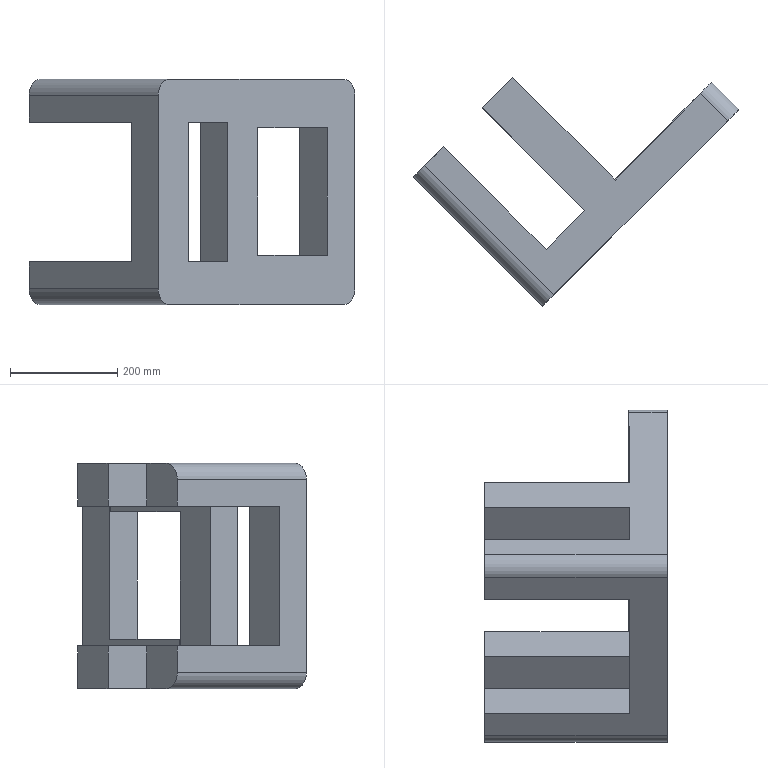Part | SolidWorks | 1 solid | 37 faces | box 606.344 x 425.772 x 420 mm | volume 17162651 mm3 | plane 33 | cylinder 4 | commonest cylinder face diameters 60 x4
STEP:
#1=CARTESIAN_POINT('',(51.005,517.696,-979.42));
#2=VERTEX_POINT('',#1);
#3=CARTESIAN_POINT('',(-139.914,708.614,-979.42));
#4=VERTEX_POINT('',#3);
#5=CARTESIAN_POINT('',(51.005,517.696,-979.42));
#6=DIRECTION('',(-0.7071,0.7071,0.));
#7=VECTOR('',#6,1000.);
#8=LINE('',#5,#7);
#9=EDGE_CURVE('',#2,#4,#8,.T.);
#10=ORIENTED_EDGE('',*,*,#9,.T.);
#11=CARTESIAN_POINT('',(-139.914,708.614,-899.42));
#12=VERTEX_POINT('',#11);
#13=CARTESIAN_POINT('',(-139.914,708.614,-899.42));
#14=DIRECTION('',(0.,0.,-1.));
#15=VECTOR('',#14,1000.);
#16=LINE('',#13,#15);
#17=EDGE_CURVE('',#12,#4,#16,.T.);
#18=ORIENTED_EDGE('',*,*,#17,.F.);
#19=CARTESIAN_POINT('',(51.005,517.696,-899.42));
#20=VERTEX_POINT('',#19);
#21=CARTESIAN_POINT('',(51.005,517.696,-899.42));
#22=DIRECTION('',(-0.7071,0.7071,0.));
#23=VECTOR('',#22,1000.);
#24=LINE('',#21,#23);
#25=EDGE_CURVE('',#20,#12,#24,.T.);
#26=ORIENTED_EDGE('',*,*,#25,.F.);
#27=CARTESIAN_POINT('',(51.005,517.696,-899.42));
#28=DIRECTION('',(0.,0.,-1.));
#29=VECTOR('',#28,1000.);
#30=LINE('',#27,#29);
#31=EDGE_CURVE('',#20,#2,#30,.T.);
#32=ORIENTED_EDGE('',*,*,#31,.T.);
#33=EDGE_LOOP('',(#10,#18,#26,#32));
#34=FACE_OUTER_BOUND('',#33,.T.);
#35=CARTESIAN_POINT('',(107.574,461.127,-1239.42));
#36=DIRECTION('',(0.7071,0.7071,0.));
#37=DIRECTION('',(0.,0.,-1.));
#38=AXIS2_PLACEMENT_3D('',#35,#36,#37);
#39=PLANE('',#38);
#40=ADVANCED_FACE('',(#34),#39,.T.);
#41=CARTESIAN_POINT('',(-196.482,652.046,-979.42));
#42=VERTEX_POINT('',#41);
#43=CARTESIAN_POINT('',(-139.914,708.614,-979.42));
#44=DIRECTION('',(-0.7071,-0.7071,0.));
#45=VECTOR('',#44,1000.);
#46=LINE('',#43,#45);
#47=EDGE_CURVE('',#4,#42,#46,.T.);
#48=ORIENTED_EDGE('',*,*,#47,.T.);
#49=CARTESIAN_POINT('',(-196.482,652.046,-899.42));
#50=VERTEX_POINT('',#49);
#51=CARTESIAN_POINT('',(-196.482,652.046,-979.42));
#52=DIRECTION('',(0.,0.,1.));
#53=VECTOR('',#52,1000.);
#54=LINE('',#51,#53);
#55=EDGE_CURVE('',#42,#50,#54,.T.);
#56=ORIENTED_EDGE('',*,*,#55,.T.);
#57=CARTESIAN_POINT('',(-196.482,652.046,-899.42));
#58=DIRECTION('',(0.7071,0.7071,0.));
#59=VECTOR('',#58,1000.);
#60=LINE('',#57,#59);
#61=EDGE_CURVE('',#50,#12,#60,.T.);
#62=ORIENTED_EDGE('',*,*,#61,.T.);
#63=ORIENTED_EDGE('',*,*,#17,.T.);
#64=EDGE_LOOP('',(#48,#56,#62,#63));
#65=FACE_OUTER_BOUND('',#64,.T.);
#66=CARTESIAN_POINT('',(-424.264,424.264,0.));
#67=DIRECTION('',(-0.7071,0.7071,0.));
#68=DIRECTION('',(-0.7071,-0.7071,0.));
#69=AXIS2_PLACEMENT_3D('',#66,#67,#68);
#70=PLANE('',#69);
#71=ADVANCED_FACE('',(#65),#70,.T.);
#72=CARTESIAN_POINT('',(-325.269,523.259,-979.42));
#73=VERTEX_POINT('',#72);
#74=CARTESIAN_POINT('',(-325.269,523.259,-929.42));
#75=VERTEX_POINT('',#74);
#76=CARTESIAN_POINT('',(-325.269,523.259,-979.42));
#77=DIRECTION('',(0.,0.,1.));
#78=VECTOR('',#77,1000.);
#79=LINE('',#76,#78);
#80=EDGE_CURVE('',#73,#75,#79,.T.);
#81=ORIENTED_EDGE('',*,*,#80,.T.);
#82=CARTESIAN_POINT('',(-304.056,544.472,-899.42));
#83=VERTEX_POINT('',#82);
#84=CARTESIAN_POINT('',(-304.056,544.472,-929.42));
#85=DIRECTION('',(-0.7071,0.7071,0.));
#86=DIRECTION('',(-0.7071,-0.7071,0.));
#87=AXIS2_PLACEMENT_3D('',#84,#85,#86);
#88=CIRCLE('',#87,30.);
#89=EDGE_CURVE('',#75,#83,#88,.T.);
#90=ORIENTED_EDGE('',*,*,#89,.T.);
#91=CARTESIAN_POINT('',(-268.701,579.828,-899.42));
#92=VERTEX_POINT('',#91);
#93=CARTESIAN_POINT('',(-325.269,523.259,-899.42));
#94=DIRECTION('',(0.7071,0.7071,0.));
#95=VECTOR('',#94,1000.);
#96=LINE('',#93,#95);
#97=EDGE_CURVE('',#83,#92,#96,.T.);
#98=ORIENTED_EDGE('',*,*,#97,.T.);
#99=CARTESIAN_POINT('',(-268.701,579.828,-979.42));
#100=VERTEX_POINT('',#99);
#101=CARTESIAN_POINT('',(-268.701,579.828,-899.42));
#102=DIRECTION('',(0.,0.,-1.));
#103=VECTOR('',#102,1000.);
#104=LINE('',#101,#103);
#105=EDGE_CURVE('',#92,#100,#104,.T.);
#106=ORIENTED_EDGE('',*,*,#105,.T.);
#107=CARTESIAN_POINT('',(-268.701,579.828,-979.42));
#108=DIRECTION('',(-0.7071,-0.7071,0.));
#109=VECTOR('',#108,1000.);
#110=LINE('',#107,#109);
#111=EDGE_CURVE('',#100,#73,#110,.T.);
#112=ORIENTED_EDGE('',*,*,#111,.T.);
#113=EDGE_LOOP('',(#81,#90,#98,#106,#112));
#114=FACE_OUTER_BOUND('',#113,.T.);
#115=CARTESIAN_POINT('',(-424.264,424.264,0.));
#116=DIRECTION('',(-0.7071,0.7071,0.));
#117=DIRECTION('',(-0.7071,-0.7071,0.));
#118=AXIS2_PLACEMENT_3D('',#115,#116,#117);
#119=PLANE('',#118);
#120=ADVANCED_FACE('',(#114),#119,.T.);
#121=CARTESIAN_POINT('',(-77.782,388.909,-979.42));
#122=VERTEX_POINT('',#121);
#123=CARTESIAN_POINT('',(-77.782,388.909,-979.42));
#124=DIRECTION('',(-0.7071,0.7071,0.));
#125=VECTOR('',#124,1000.);
#126=LINE('',#123,#125);
#127=EDGE_CURVE('',#122,#100,#126,.T.);
#128=ORIENTED_EDGE('',*,*,#127,.T.);
#129=ORIENTED_EDGE('',*,*,#105,.F.);
#130=CARTESIAN_POINT('',(-77.782,388.909,-899.42));
#131=VERTEX_POINT('',#130);
#132=CARTESIAN_POINT('',(-77.782,388.909,-899.42));
#133=DIRECTION('',(-0.7071,0.7071,0.));
#134=VECTOR('',#133,1000.);
#135=LINE('',#132,#134);
#136=EDGE_CURVE('',#131,#92,#135,.T.);
#137=ORIENTED_EDGE('',*,*,#136,.F.);
#138=CARTESIAN_POINT('',(-77.782,388.909,-899.42));
#139=DIRECTION('',(0.,0.,-1.));
#140=VECTOR('',#139,1000.);
#141=LINE('',#138,#140);
#142=EDGE_CURVE('',#131,#122,#141,.T.);
#143=ORIENTED_EDGE('',*,*,#142,.T.);
#144=EDGE_LOOP('',(#128,#129,#137,#143));
#145=FACE_OUTER_BOUND('',#144,.T.);
#146=CARTESIAN_POINT('',(-28.284,339.411,-899.42));
#147=DIRECTION('',(0.7071,0.7071,0.));
#148=DIRECTION('',(0.,0.,-1.));
#149=AXIS2_PLACEMENT_3D('',#146,#147,#148);
#150=PLANE('',#149);
#151=ADVANCED_FACE('',(#145),#150,.T.);
#152=CARTESIAN_POINT('',(-134.35,332.34,-979.42));
#153=VERTEX_POINT('',#152);
#154=CARTESIAN_POINT('',(-77.782,388.909,-979.42));
#155=DIRECTION('',(-0.7071,-0.7071,0.));
#156=VECTOR('',#155,1000.);
#157=LINE('',#154,#156);
#158=EDGE_CURVE('',#122,#153,#157,.T.);
#159=ORIENTED_EDGE('',*,*,#158,.T.);
#160=CARTESIAN_POINT('',(-134.35,332.34,-979.42));
#161=DIRECTION('',(-0.7071,0.7071,0.));
#162=VECTOR('',#161,1000.);
#163=LINE('',#160,#162);
#164=EDGE_CURVE('',#153,#73,#163,.T.);
#165=ORIENTED_EDGE('',*,*,#164,.T.);
#166=ORIENTED_EDGE('',*,*,#111,.F.);
#167=ORIENTED_EDGE('',*,*,#127,.F.);
#168=EDGE_LOOP('',(#159,#165,#166,#167));
#169=FACE_OUTER_BOUND('',#168,.T.);
#170=CARTESIAN_POINT('',(-28.284,339.411,-979.42));
#171=DIRECTION('',(0.,0.,-1.));
#172=DIRECTION('',(-0.7071,-0.7071,0.));
#173=AXIS2_PLACEMENT_3D('',#170,#171,#172);
#174=PLANE('',#173);
#175=ADVANCED_FACE('',(#169),#174,.T.);
#176=CARTESIAN_POINT('',(-134.35,332.34,-1239.42));
#177=VERTEX_POINT('',#176);
#178=CARTESIAN_POINT('',(-77.782,388.909,-1239.42));
#179=VERTEX_POINT('',#178);
#180=CARTESIAN_POINT('',(-134.35,332.34,-1239.42));
#181=DIRECTION('',(0.7071,0.7071,0.));
#182=VECTOR('',#181,1000.);
#183=LINE('',#180,#182);
#184=EDGE_CURVE('',#177,#179,#183,.T.);
#185=ORIENTED_EDGE('',*,*,#184,.F.);
#186=CARTESIAN_POINT('',(-134.35,332.34,-1239.42));
#187=DIRECTION('',(0.,0.,1.));
#188=VECTOR('',#187,1000.);
#189=LINE('',#186,#188);
#190=EDGE_CURVE('',#177,#153,#189,.T.);
#191=ORIENTED_EDGE('',*,*,#190,.T.);
#192=ORIENTED_EDGE('',*,*,#158,.F.);
#193=CARTESIAN_POINT('',(-77.782,388.909,-1239.42));
#194=DIRECTION('',(0.,0.,1.));
#195=VECTOR('',#194,1000.);
#196=LINE('',#193,#195);
#197=EDGE_CURVE('',#179,#122,#196,.T.);
#198=ORIENTED_EDGE('',*,*,#197,.F.);
#199=EDGE_LOOP('',(#185,#191,#192,#198));
#200=FACE_OUTER_BOUND('',#199,.T.);
#201=CARTESIAN_POINT('',(-134.35,332.34,-1319.42));
#202=DIRECTION('',(-0.7071,0.7071,0.));
#203=DIRECTION('',(0.7071,0.7071,0.));
#204=AXIS2_PLACEMENT_3D('',#201,#202,#203);
#205=PLANE('',#204);
#206=ADVANCED_FACE('',(#200),#205,.T.);
#207=CARTESIAN_POINT('',(43.934,411.63,-979.42));
#208=VERTEX_POINT('',#207);
#209=CARTESIAN_POINT('',(-5.563,461.127,-979.42));
#210=VERTEX_POINT('',#209);
#211=CARTESIAN_POINT('',(43.934,411.63,-979.42));
#212=DIRECTION('',(-0.7071,0.7071,0.));
#213=VECTOR('',#212,1000.);
#214=LINE('',#211,#213);
#215=EDGE_CURVE('',#208,#210,#214,.T.);
#216=ORIENTED_EDGE('',*,*,#215,.T.);
#217=CARTESIAN_POINT('',(-5.563,461.127,-1239.42));
#218=VERTEX_POINT('',#217);
#219=CARTESIAN_POINT('',(-5.563,461.127,-1239.42));
#220=DIRECTION('',(0.,0.,1.));
#221=VECTOR('',#220,1000.);
#222=LINE('',#219,#221);
#223=EDGE_CURVE('',#218,#210,#222,.T.);
#224=ORIENTED_EDGE('',*,*,#223,.F.);
#225=CARTESIAN_POINT('',(43.934,411.63,-1239.42));
#226=VERTEX_POINT('',#225);
#227=CARTESIAN_POINT('',(43.934,411.63,-1239.42));
#228=DIRECTION('',(-0.7071,0.7071,0.));
#229=VECTOR('',#228,1000.);
#230=LINE('',#227,#229);
#231=EDGE_CURVE('',#226,#218,#230,.T.);
#232=ORIENTED_EDGE('',*,*,#231,.F.);
#233=CARTESIAN_POINT('',(43.934,411.63,-1239.42));
#234=DIRECTION('',(0.,0.,1.));
#235=VECTOR('',#234,1000.);
#236=LINE('',#233,#235);
#237=EDGE_CURVE('',#226,#208,#236,.T.);
#238=ORIENTED_EDGE('',*,*,#237,.T.);
#239=EDGE_LOOP('',(#216,#224,#232,#238));
#240=FACE_OUTER_BOUND('',#239,.T.);
#241=CARTESIAN_POINT('',(51.005,404.558,-1319.42));
#242=DIRECTION('',(-0.7071,-0.7071,0.));
#243=DIRECTION('',(0.,0.,1.));
#244=AXIS2_PLACEMENT_3D('',#241,#242,#243);
#245=PLANE('',#244);
#246=ADVANCED_FACE('',(#240),#245,.T.);
#247=CARTESIAN_POINT('',(-28.284,339.411,-979.42));
#248=VERTEX_POINT('',#247);
#249=CARTESIAN_POINT('',(-28.284,339.411,-979.42));
#250=DIRECTION('',(-0.7071,0.7071,0.));
#251=VECTOR('',#250,1000.);
#252=LINE('',#249,#251);
#253=EDGE_CURVE('',#248,#122,#252,.T.);
#254=ORIENTED_EDGE('',*,*,#253,.T.);
#255=CARTESIAN_POINT('',(-77.782,388.909,-979.42));
#256=DIRECTION('',(0.7071,0.7071,0.));
#257=VECTOR('',#256,1000.);
#258=LINE('',#255,#257);
#259=EDGE_CURVE('',#122,#210,#258,.T.);
#260=ORIENTED_EDGE('',*,*,#259,.T.);
#261=ORIENTED_EDGE('',*,*,#215,.F.);
#262=CARTESIAN_POINT('',(43.934,411.63,-979.42));
#263=DIRECTION('',(-0.7071,-0.7071,0.));
#264=VECTOR('',#263,1000.);
#265=LINE('',#262,#264);
#266=EDGE_CURVE('',#208,#248,#265,.T.);
#267=ORIENTED_EDGE('',*,*,#266,.T.);
#268=EDGE_LOOP('',(#254,#260,#261,#267));
#269=FACE_OUTER_BOUND('',#268,.T.);
#270=CARTESIAN_POINT('',(-134.35,332.34,-979.42));
#271=DIRECTION('',(0.,0.,-1.));
#272=DIRECTION('',(0.7071,-0.7071,0.));
#273=AXIS2_PLACEMENT_3D('',#270,#271,#272);
#274=PLANE('',#273);
#275=ADVANCED_FACE('',(#269),#274,.T.);
#276=CARTESIAN_POINT('',(-28.284,339.411,-1239.42));
#277=VERTEX_POINT('',#276);
#278=CARTESIAN_POINT('',(-28.284,339.411,-1239.42));
#279=DIRECTION('',(-0.7071,0.7071,0.));
#280=VECTOR('',#279,1000.);
#281=LINE('',#278,#280);
#282=EDGE_CURVE('',#277,#179,#281,.T.);
#283=ORIENTED_EDGE('',*,*,#282,.T.);
#284=ORIENTED_EDGE('',*,*,#197,.T.);
#285=ORIENTED_EDGE('',*,*,#253,.F.);
#286=CARTESIAN_POINT('',(-28.284,339.411,-979.42));
#287=DIRECTION('',(0.,0.,-1.));
#288=VECTOR('',#287,1000.);
#289=LINE('',#286,#288);
#290=EDGE_CURVE('',#248,#277,#289,.T.);
#291=ORIENTED_EDGE('',*,*,#290,.T.);
#292=EDGE_LOOP('',(#283,#284,#285,#291));
#293=FACE_OUTER_BOUND('',#292,.T.);
#294=CARTESIAN_POINT('',(-28.284,339.411,-899.42));
#295=DIRECTION('',(0.7071,0.7071,0.));
#296=DIRECTION('',(0.,0.,-1.));
#297=AXIS2_PLACEMENT_3D('',#294,#295,#296);
#298=PLANE('',#297);
#299=ADVANCED_FACE('',(#293),#298,.T.);
#300=ORIENTED_EDGE('',*,*,#231,.T.);
#301=CARTESIAN_POINT('',(-77.782,388.909,-1239.42));
#302=DIRECTION('',(0.7071,0.7071,0.));
#303=VECTOR('',#302,1000.);
#304=LINE('',#301,#303);
#305=EDGE_CURVE('',#179,#218,#304,.T.);
#306=ORIENTED_EDGE('',*,*,#305,.F.);
#307=ORIENTED_EDGE('',*,*,#282,.F.);
#308=CARTESIAN_POINT('',(43.934,411.63,-1239.42));
#309=DIRECTION('',(-0.7071,-0.7071,0.));
#310=VECTOR('',#309,1000.);
#311=LINE('',#308,#310);
#312=EDGE_CURVE('',#226,#277,#311,.T.);
#313=ORIENTED_EDGE('',*,*,#312,.F.);
#314=EDGE_LOOP('',(#300,#306,#307,#313));
#315=FACE_OUTER_BOUND('',#314,.T.);
#316=CARTESIAN_POINT('',(-77.782,275.772,-1239.42));
#317=DIRECTION('',(0.,0.,1.));
#318=DIRECTION('',(-0.7071,0.7071,0.));
#319=AXIS2_PLACEMENT_3D('',#316,#317,#318);
#320=PLANE('',#319);
#321=ADVANCED_FACE('',(#315),#320,.T.);
#322=CARTESIAN_POINT('',(49.428,519.273,-1239.42));
#323=VERTEX_POINT('',#322);
#324=CARTESIAN_POINT('',(-139.914,708.614,-1239.42));
#325=VERTEX_POINT('',#324);
#326=CARTESIAN_POINT('',(49.428,519.273,-1239.42));
#327=DIRECTION('',(-0.7071,0.7071,0.));
#328=VECTOR('',#327,1000.);
#329=LINE('',#326,#328);
#330=EDGE_CURVE('',#323,#325,#329,.T.);
#331=ORIENTED_EDGE('',*,*,#330,.T.);
#332=CARTESIAN_POINT('',(-196.482,652.046,-1239.42));
#333=VERTEX_POINT('',#332);
#334=CARTESIAN_POINT('',(-196.482,652.046,-1239.42));
#335=DIRECTION('',(0.7071,0.7071,0.));
#336=VECTOR('',#335,1000.);
#337=LINE('',#334,#336);
#338=EDGE_CURVE('',#333,#325,#337,.T.);
#339=ORIENTED_EDGE('',*,*,#338,.F.);
#340=CARTESIAN_POINT('',(-5.563,461.127,-1239.42));
#341=DIRECTION('',(-0.7071,0.7071,0.));
#342=VECTOR('',#341,1000.);
#343=LINE('',#340,#342);
#344=EDGE_CURVE('',#218,#333,#343,.T.);
#345=ORIENTED_EDGE('',*,*,#344,.F.);
#346=CARTESIAN_POINT('',(51.005,517.696,-1239.42));
#347=VERTEX_POINT('',#346);
#348=CARTESIAN_POINT('',(-5.563,461.127,-1239.42));
#349=DIRECTION('',(0.7071,0.7071,0.));
#350=VECTOR('',#349,1000.);
#351=LINE('',#348,#350);
#352=EDGE_CURVE('',#218,#347,#351,.T.);
#353=ORIENTED_EDGE('',*,*,#352,.T.);
#354=CARTESIAN_POINT('',(51.005,517.696,-1239.42));
#355=DIRECTION('',(-0.7071,0.7071,0.));
#356=VECTOR('',#355,1000.);
#357=LINE('',#354,#356);
#358=EDGE_CURVE('',#347,#323,#357,.T.);
#359=ORIENTED_EDGE('',*,*,#358,.T.);
#360=EDGE_LOOP('',(#331,#339,#345,#353,#359));
#361=FACE_OUTER_BOUND('',#360,.T.);
#362=CARTESIAN_POINT('',(51.005,404.558,-1239.42));
#363=DIRECTION('',(0.,0.,1.));
#364=DIRECTION('',(0.7071,0.7071,0.));
#365=AXIS2_PLACEMENT_3D('',#362,#363,#364);
#366=PLANE('',#365);
#367=ADVANCED_FACE('',(#361),#366,.T.);
#368=CARTESIAN_POINT('',(51.005,517.696,-1227.42));
#369=VERTEX_POINT('',#368);
#370=CARTESIAN_POINT('',(51.005,517.696,-1227.42));
#371=DIRECTION('',(0.,0.,-1.));
#372=VECTOR('',#371,1000.);
#373=LINE('',#370,#372);
#374=EDGE_CURVE('',#369,#347,#373,.T.);
#375=ORIENTED_EDGE('',*,*,#374,.F.);
#376=CARTESIAN_POINT('',(49.428,519.273,-1227.42));
#377=VERTEX_POINT('',#376);
#378=CARTESIAN_POINT('',(49.428,519.273,-1227.42));
#379=DIRECTION('',(0.7071,-0.7071,0.));
#380=VECTOR('',#379,1000.);
#381=LINE('',#378,#380);
#382=EDGE_CURVE('',#377,#369,#381,.T.);
#383=ORIENTED_EDGE('',*,*,#382,.F.);
#384=CARTESIAN_POINT('',(49.428,519.273,-1239.42));
#385=DIRECTION('',(0.,0.,1.));
#386=VECTOR('',#385,1000.);
#387=LINE('',#384,#386);
#388=EDGE_CURVE('',#323,#377,#387,.T.);
#389=ORIENTED_EDGE('',*,*,#388,.F.);
#390=ORIENTED_EDGE('',*,*,#358,.F.);
#391=EDGE_LOOP('',(#375,#383,#389,#390));
#392=FACE_OUTER_BOUND('',#391,.T.);
#393=CARTESIAN_POINT('',(107.574,461.127,0.));
#394=DIRECTION('',(0.7071,0.7071,0.));
#395=DIRECTION('',(0.,0.,1.));
#396=AXIS2_PLACEMENT_3D('',#393,#394,#395);
#397=PLANE('',#396);
#398=ADVANCED_FACE('',(#392),#397,.F.);
#399=CARTESIAN_POINT('',(100.503,468.198,-1227.42));
#400=VERTEX_POINT('',#399);
#401=CARTESIAN_POINT('',(230.,597.696,-1227.42));
#402=VERTEX_POINT('',#401);
#403=CARTESIAN_POINT('',(100.503,468.198,-1227.42));
#404=DIRECTION('',(0.7071,0.7071,0.));
#405=VECTOR('',#404,1000.);
#406=LINE('',#403,#405);
#407=EDGE_CURVE('',#400,#402,#406,.T.);
#408=ORIENTED_EDGE('',*,*,#407,.T.);
#409=CARTESIAN_POINT('',(178.925,648.77,-1227.42));
#410=VERTEX_POINT('',#409);
#411=CARTESIAN_POINT('',(178.925,648.77,-1227.42));
#412=DIRECTION('',(0.7071,-0.7071,0.));
#413=VECTOR('',#412,1000.);
#414=LINE('',#411,#413);
#415=EDGE_CURVE('',#410,#402,#414,.T.);
#416=ORIENTED_EDGE('',*,*,#415,.F.);
#417=CARTESIAN_POINT('',(49.428,519.273,-1227.42));
#418=DIRECTION('',(0.7071,0.7071,0.));
#419=VECTOR('',#418,1000.);
#420=LINE('',#417,#419);
#421=EDGE_CURVE('',#377,#410,#420,.T.);
#422=ORIENTED_EDGE('',*,*,#421,.F.);
#423=ORIENTED_EDGE('',*,*,#382,.T.);
#424=CARTESIAN_POINT('',(51.005,517.696,-1227.42));
#425=DIRECTION('',(0.7071,-0.7071,0.));
#426=VECTOR('',#425,1000.);
#427=LINE('',#424,#426);
#428=EDGE_CURVE('',#369,#400,#427,.T.);
#429=ORIENTED_EDGE('',*,*,#428,.T.);
#430=EDGE_LOOP('',(#408,#416,#422,#423,#429));
#431=FACE_OUTER_BOUND('',#430,.T.);
#432=CARTESIAN_POINT('',(49.428,519.273,-1227.42));
#433=DIRECTION('',(0.,0.,1.));
#434=DIRECTION('',(0.7071,-0.7071,0.));
#435=AXIS2_PLACEMENT_3D('',#432,#433,#434);
#436=PLANE('',#435);
#437=ADVANCED_FACE('',(#431),#436,.T.);
#438=CARTESIAN_POINT('',(230.,699.845,-1289.42));
#439=VERTEX_POINT('',#438);
#440=CARTESIAN_POINT('',(230.,699.845,-929.42));
#441=VERTEX_POINT('',#440);
#442=CARTESIAN_POINT('',(230.,699.845,-1319.42));
#443=DIRECTION('',(0.,0.,1.));
#444=VECTOR('',#443,1000.);
#445=LINE('',#442,#444);
#446=EDGE_CURVE('',#439,#441,#445,.T.);
#447=ORIENTED_EDGE('',*,*,#446,.F.);
#448=CARTESIAN_POINT('',(208.787,678.632,-1319.42));
#449=VERTEX_POINT('',#448);
#450=CARTESIAN_POINT('',(208.787,678.632,-1289.42));
#451=DIRECTION('',(-0.7071,0.7071,0.));
#452=DIRECTION('',(-0.7071,-0.7071,0.));
#453=AXIS2_PLACEMENT_3D('',#450,#451,#452);
#454=CIRCLE('',#453,30.);
#455=EDGE_CURVE('',#439,#449,#454,.T.);
#456=ORIENTED_EDGE('',*,*,#455,.T.);
#457=CARTESIAN_POINT('',(49.428,519.273,-1319.42));
#458=VERTEX_POINT('',#457);
#459=CARTESIAN_POINT('',(49.428,519.273,-1319.42));
#460=DIRECTION('',(0.7071,0.7071,0.));
#461=VECTOR('',#460,1000.);
#462=LINE('',#459,#461);
#463=EDGE_CURVE('',#458,#449,#462,.T.);
#464=ORIENTED_EDGE('',*,*,#463,.F.);
#465=CARTESIAN_POINT('',(49.428,519.273,-1319.42));
#466=DIRECTION('',(0.,0.,1.));
#467=VECTOR('',#466,1000.);
#468=LINE('',#465,#467);
#469=EDGE_CURVE('',#458,#323,#468,.T.);
#470=ORIENTED_EDGE('',*,*,#469,.T.);
#471=ORIENTED_EDGE('',*,*,#388,.T.);
#472=ORIENTED_EDGE('',*,*,#421,.T.);
#473=CARTESIAN_POINT('',(178.925,648.77,-899.42));
#474=VERTEX_POINT('',#473);
#475=CARTESIAN_POINT('',(178.925,648.77,-1227.42));
#476=DIRECTION('',(0.,0.,1.));
#477=VECTOR('',#476,1000.);
#478=LINE('',#475,#477);
#479=EDGE_CURVE('',#410,#474,#478,.T.);
#480=ORIENTED_EDGE('',*,*,#479,.T.);
#481=CARTESIAN_POINT('',(208.787,678.632,-899.42));
#482=VERTEX_POINT('',#481);
#483=CARTESIAN_POINT('',(178.925,648.77,-899.42));
#484=DIRECTION('',(0.7071,0.7071,0.));
#485=VECTOR('',#484,1000.);
#486=LINE('',#483,#485);
#487=EDGE_CURVE('',#474,#482,#486,.T.);
#488=ORIENTED_EDGE('',*,*,#487,.T.);
#489=CARTESIAN_POINT('',(208.787,678.632,-929.42));
#490=DIRECTION('',(-0.7071,0.7071,0.));
#491=DIRECTION('',(-0.7071,-0.7071,0.));
#492=AXIS2_PLACEMENT_3D('',#489,#490,#491);
#493=CIRCLE('',#492,30.);
#494=EDGE_CURVE('',#482,#441,#493,.T.);
#495=ORIENTED_EDGE('',*,*,#494,.T.);
#496=EDGE_LOOP('',(#447,#456,#464,#470,#471,#472,#480,#488,#495));
#497=FACE_OUTER_BOUND('',#496,.T.);
#498=CARTESIAN_POINT('',(49.428,519.273,-1319.42));
#499=DIRECTION('',(-0.7071,0.7071,0.));
#500=DIRECTION('',(0.,0.,1.));
#501=AXIS2_PLACEMENT_3D('',#498,#499,#500);
#502=PLANE('',#501);
#503=ADVANCED_FACE('',(#497),#502,.T.);
#504=CARTESIAN_POINT('',(-139.914,708.614,-1319.42));
#505=VERTEX_POINT('',#504);
#506=CARTESIAN_POINT('',(49.428,519.273,-1319.42));
#507=DIRECTION('',(-0.7071,0.7071,0.));
#508=VECTOR('',#507,1000.);
#509=LINE('',#506,#508);
#510=EDGE_CURVE('',#458,#505,#509,.T.);
#511=ORIENTED_EDGE('',*,*,#510,.T.);
#512=CARTESIAN_POINT('',(-139.914,708.614,-1239.42));
#513=DIRECTION('',(0.,0.,-1.));
#514=VECTOR('',#513,1000.);
#515=LINE('',#512,#514);
#516=EDGE_CURVE('',#325,#505,#515,.T.);
#517=ORIENTED_EDGE('',*,*,#516,.F.);
#518=ORIENTED_EDGE('',*,*,#330,.F.);
#519=ORIENTED_EDGE('',*,*,#469,.F.);
#520=EDGE_LOOP('',(#511,#517,#518,#519));
#521=FACE_OUTER_BOUND('',#520,.T.);
#522=CARTESIAN_POINT('',(107.574,461.127,-1239.42));
#523=DIRECTION('',(0.7071,0.7071,0.));
#524=DIRECTION('',(0.,0.,-1.));
#525=AXIS2_PLACEMENT_3D('',#522,#523,#524);
#526=PLANE('',#525);
#527=ADVANCED_FACE('',(#521),#526,.T.);
#528=CARTESIAN_POINT('',(-196.482,652.046,-1319.42));
#529=VERTEX_POINT('',#528);
#530=CARTESIAN_POINT('',(-196.482,652.046,-1319.42));
#531=DIRECTION('',(0.,0.,1.));
#532=VECTOR('',#531,1000.);
#533=LINE('',#530,#532);
#534=EDGE_CURVE('',#529,#333,#533,.T.);
#535=ORIENTED_EDGE('',*,*,#534,.T.);
#536=ORIENTED_EDGE('',*,*,#338,.T.);
#537=ORIENTED_EDGE('',*,*,#516,.T.);
#538=CARTESIAN_POINT('',(-139.914,708.614,-1319.42));
#539=DIRECTION('',(-0.7071,-0.7071,0.));
#540=VECTOR('',#539,1000.);
#541=LINE('',#538,#540);
#542=EDGE_CURVE('',#505,#529,#541,.T.);
#543=ORIENTED_EDGE('',*,*,#542,.T.);
#544=EDGE_LOOP('',(#535,#536,#537,#543));
#545=FACE_OUTER_BOUND('',#544,.T.);
#546=CARTESIAN_POINT('',(-424.264,424.264,0.));
#547=DIRECTION('',(-0.7071,0.7071,0.));
#548=DIRECTION('',(-0.7071,-0.7071,0.));
#549=AXIS2_PLACEMENT_3D('',#546,#547,#548);
#550=PLANE('',#549);
#551=ADVANCED_FACE('',(#545),#550,.T.);
#552=ORIENTED_EDGE('',*,*,#344,.T.);
#553=ORIENTED_EDGE('',*,*,#534,.F.);
#554=CARTESIAN_POINT('',(-5.563,461.127,-1319.42));
#555=VERTEX_POINT('',#554);
#556=CARTESIAN_POINT('',(-5.563,461.127,-1319.42));
#557=DIRECTION('',(-0.7071,0.7071,0.));
#558=VECTOR('',#557,1000.);
#559=LINE('',#556,#558);
#560=EDGE_CURVE('',#555,#529,#559,.T.);
#561=ORIENTED_EDGE('',*,*,#560,.F.);
#562=CARTESIAN_POINT('',(-5.563,461.127,-1319.42));
#563=DIRECTION('',(0.,0.,1.));
#564=VECTOR('',#563,1000.);
#565=LINE('',#562,#564);
#566=EDGE_CURVE('',#555,#218,#565,.T.);
#567=ORIENTED_EDGE('',*,*,#566,.T.);
#568=EDGE_LOOP('',(#552,#553,#561,#567));
#569=FACE_OUTER_BOUND('',#568,.T.);
#570=CARTESIAN_POINT('',(51.005,404.558,-1319.42));
#571=DIRECTION('',(-0.7071,-0.7071,0.));
#572=DIRECTION('',(0.,0.,1.));
#573=AXIS2_PLACEMENT_3D('',#570,#571,#572);
#574=PLANE('',#573);
#575=ADVANCED_FACE('',(#569),#574,.T.);
#576=CARTESIAN_POINT('',(-77.782,388.909,-1319.42));
#577=VERTEX_POINT('',#576);
#578=CARTESIAN_POINT('',(-77.782,388.909,-1319.42));
#579=DIRECTION('',(0.7071,0.7071,0.));
#580=VECTOR('',#579,1000.);
#581=LINE('',#578,#580);
#582=EDGE_CURVE('',#577,#555,#581,.T.);
#583=ORIENTED_EDGE('',*,*,#582,.F.);
#584=CARTESIAN_POINT('',(-77.782,388.909,-1319.42));
#585=DIRECTION('',(0.,0.,1.));
#586=VECTOR('',#585,1000.);
#587=LINE('',#584,#586);
#588=EDGE_CURVE('',#577,#179,#587,.T.);
#589=ORIENTED_EDGE('',*,*,#588,.T.);
#590=ORIENTED_EDGE('',*,*,#305,.T.);
#591=ORIENTED_EDGE('',*,*,#566,.F.);
#592=EDGE_LOOP('',(#583,#589,#590,#591));
#593=FACE_OUTER_BOUND('',#592,.T.);
#594=CARTESIAN_POINT('',(-134.35,332.34,-1239.42));
#595=DIRECTION('',(-0.7071,0.7071,0.));
#596=DIRECTION('',(0.,0.,-1.));
#597=AXIS2_PLACEMENT_3D('',#594,#595,#596);
#598=PLANE('',#597);
#599=ADVANCED_FACE('',(#593),#598,.T.);
#600=CARTESIAN_POINT('',(-268.701,579.828,-1319.42));
#601=VERTEX_POINT('',#600);
#602=CARTESIAN_POINT('',(-268.701,579.828,-1319.42));
#603=DIRECTION('',(0.7071,-0.7071,0.));
#604=VECTOR('',#603,1000.);
#605=LINE('',#602,#604);
#606=EDGE_CURVE('',#601,#577,#605,.T.);
#607=ORIENTED_EDGE('',*,*,#606,.F.);
#608=CARTESIAN_POINT('',(-268.701,579.828,-1239.42));
#609=VERTEX_POINT('',#608);
#610=CARTESIAN_POINT('',(-268.701,579.828,-1239.42));
#611=DIRECTION('',(0.,0.,-1.));
#612=VECTOR('',#611,1000.);
#613=LINE('',#610,#612);
#614=EDGE_CURVE('',#609,#601,#613,.T.);
#615=ORIENTED_EDGE('',*,*,#614,.F.);
#616=CARTESIAN_POINT('',(-77.782,388.909,-1239.42));
#617=DIRECTION('',(-0.7071,0.7071,0.));
#618=VECTOR('',#617,1000.);
#619=LINE('',#616,#618);
#620=EDGE_CURVE('',#179,#609,#619,.T.);
#621=ORIENTED_EDGE('',*,*,#620,.F.);
#622=ORIENTED_EDGE('',*,*,#588,.F.);
#623=EDGE_LOOP('',(#607,#615,#621,#622));
#624=FACE_OUTER_BOUND('',#623,.T.);
#625=CARTESIAN_POINT('',(-28.284,339.411,-899.42));
#626=DIRECTION('',(0.7071,0.7071,0.));
#627=DIRECTION('',(0.,0.,-1.));
#628=AXIS2_PLACEMENT_3D('',#625,#626,#627);
#629=PLANE('',#628);
#630=ADVANCED_FACE('',(#624),#629,.T.);
#631=CARTESIAN_POINT('',(-325.269,523.259,-1239.42));
#632=VERTEX_POINT('',#631);
#633=CARTESIAN_POINT('',(-325.269,523.259,-1239.42));
#634=DIRECTION('',(0.7071,0.7071,0.));
#635=VECTOR('',#634,1000.);
#636=LINE('',#633,#635);
#637=EDGE_CURVE('',#632,#609,#636,.T.);
#638=ORIENTED_EDGE('',*,*,#637,.F.);
#639=CARTESIAN_POINT('',(-134.35,332.34,-1239.42));
#640=DIRECTION('',(-0.7071,0.7071,0.));
#641=VECTOR('',#640,1000.);
#642=LINE('',#639,#641);
#643=EDGE_CURVE('',#177,#632,#642,.T.);
#644=ORIENTED_EDGE('',*,*,#643,.F.);
#645=ORIENTED_EDGE('',*,*,#184,.T.);
#646=ORIENTED_EDGE('',*,*,#620,.T.);
#647=EDGE_LOOP('',(#638,#644,#645,#646));
#648=FACE_OUTER_BOUND('',#647,.T.);
#649=CARTESIAN_POINT('',(-84.853,282.843,-1239.42));
#650=DIRECTION('',(0.,0.,1.));
#651=DIRECTION('',(0.7071,0.7071,0.));
#652=AXIS2_PLACEMENT_3D('',#649,#650,#651);
#653=PLANE('',#652);
#654=ADVANCED_FACE('',(#648),#653,.T.);
#655=CARTESIAN_POINT('',(-304.056,544.472,-1319.42));
#656=VERTEX_POINT('',#655);
#657=CARTESIAN_POINT('',(-268.701,579.828,-1319.42));
#658=DIRECTION('',(-0.7071,-0.7071,0.));
#659=VECTOR('',#658,1000.);
#660=LINE('',#657,#659);
#661=EDGE_CURVE('',#601,#656,#660,.T.);
#662=ORIENTED_EDGE('',*,*,#661,.T.);
#663=CARTESIAN_POINT('',(-325.269,523.259,-1289.42));
#664=VERTEX_POINT('',#663);
#665=CARTESIAN_POINT('',(-304.056,544.472,-1289.42));
#666=DIRECTION('',(-0.7071,0.7071,0.));
#667=DIRECTION('',(-0.7071,-0.7071,0.));
#668=AXIS2_PLACEMENT_3D('',#665,#666,#667);
#669=CIRCLE('',#668,30.);
#670=EDGE_CURVE('',#656,#664,#669,.T.);
#671=ORIENTED_EDGE('',*,*,#670,.T.);
#672=CARTESIAN_POINT('',(-325.269,523.259,-1319.42));
#673=DIRECTION('',(0.,0.,1.));
#674=VECTOR('',#673,1000.);
#675=LINE('',#672,#674);
#676=EDGE_CURVE('',#664,#632,#675,.T.);
#677=ORIENTED_EDGE('',*,*,#676,.T.);
#678=ORIENTED_EDGE('',*,*,#637,.T.);
#679=ORIENTED_EDGE('',*,*,#614,.T.);
#680=EDGE_LOOP('',(#662,#671,#677,#678,#679));
#681=FACE_OUTER_BOUND('',#680,.T.);
#682=CARTESIAN_POINT('',(-424.264,424.264,0.));
#683=DIRECTION('',(-0.7071,0.7071,0.));
#684=DIRECTION('',(-0.7071,-0.7071,0.));
#685=AXIS2_PLACEMENT_3D('',#682,#683,#684);
#686=PLANE('',#685);
#687=ADVANCED_FACE('',(#681),#686,.T.);
#688=ORIENTED_EDGE('',*,*,#676,.F.);
#689=CARTESIAN_POINT('',(-84.853,282.843,-1289.42));
#690=VERTEX_POINT('',#689);
#691=CARTESIAN_POINT('',(-84.853,282.843,-1289.42));
#692=DIRECTION('',(0.7071,-0.7071,0.));
#693=VECTOR('',#692,1000.);
#694=LINE('',#691,#693);
#695=EDGE_CURVE('',#664,#690,#694,.T.);
#696=ORIENTED_EDGE('',*,*,#695,.T.);
#697=CARTESIAN_POINT('',(-84.853,282.843,-929.42));
#698=VERTEX_POINT('',#697);
#699=CARTESIAN_POINT('',(-84.853,282.843,-1319.42));
#700=DIRECTION('',(0.,0.,1.));
#701=VECTOR('',#700,1000.);
#702=LINE('',#699,#701);
#703=EDGE_CURVE('',#690,#698,#702,.T.);
#704=ORIENTED_EDGE('',*,*,#703,.T.);
#705=CARTESIAN_POINT('',(-84.853,282.843,-929.42));
#706=DIRECTION('',(-0.7071,0.7071,0.));
#707=VECTOR('',#706,1000.);
#708=LINE('',#705,#707);
#709=EDGE_CURVE('',#698,#75,#708,.T.);
#710=ORIENTED_EDGE('',*,*,#709,.T.);
#711=ORIENTED_EDGE('',*,*,#80,.F.);
#712=ORIENTED_EDGE('',*,*,#164,.F.);
#713=ORIENTED_EDGE('',*,*,#190,.F.);
#714=ORIENTED_EDGE('',*,*,#643,.T.);
#715=EDGE_LOOP('',(#688,#696,#704,#710,#711,#712,#713,#714));
#716=FACE_OUTER_BOUND('',#715,.T.);
#717=CARTESIAN_POINT('',(-84.853,282.843,-979.42));
#718=DIRECTION('',(-0.7071,-0.7071,0.));
#719=DIRECTION('',(0.,0.,1.));
#720=AXIS2_PLACEMENT_3D('',#717,#718,#719);
#721=PLANE('',#720);
#722=ADVANCED_FACE('',(#716),#721,.T.);
#723=ORIENTED_EDGE('',*,*,#97,.F.);
#724=CARTESIAN_POINT('',(-63.64,304.056,-899.42));
#725=VERTEX_POINT('',#724);
#726=CARTESIAN_POINT('',(-56.569,296.985,-899.42));
#727=DIRECTION('',(0.7071,-0.7071,0.));
#728=VECTOR('',#727,1000.);
#729=LINE('',#726,#728);
#730=EDGE_CURVE('',#83,#725,#729,.T.);
#731=ORIENTED_EDGE('',*,*,#730,.T.);
#732=CARTESIAN_POINT('',(259.862,627.557,-899.42));
#733=VERTEX_POINT('',#732);
#734=CARTESIAN_POINT('',(-84.853,282.843,-899.42));
#735=DIRECTION('',(0.7071,0.7071,0.));
#736=VECTOR('',#735,1000.);
#737=LINE('',#734,#736);
#738=EDGE_CURVE('',#725,#733,#737,.T.);
#739=ORIENTED_EDGE('',*,*,#738,.T.);
#740=CARTESIAN_POINT('',(266.933,620.486,-899.42));
#741=DIRECTION('',(-0.7071,0.7071,0.));
#742=VECTOR('',#741,1000.);
#743=LINE('',#740,#742);
#744=EDGE_CURVE('',#733,#482,#743,.T.);
#745=ORIENTED_EDGE('',*,*,#744,.T.);
#746=ORIENTED_EDGE('',*,*,#487,.F.);
#747=CARTESIAN_POINT('',(180.503,647.193,-899.42));
#748=VERTEX_POINT('',#747);
#749=CARTESIAN_POINT('',(180.503,647.193,-899.42));
#750=DIRECTION('',(-0.7071,0.7071,0.));
#751=VECTOR('',#750,1000.);
#752=LINE('',#749,#751);
#753=EDGE_CURVE('',#748,#474,#752,.T.);
#754=ORIENTED_EDGE('',*,*,#753,.F.);
#755=CARTESIAN_POINT('',(51.005,517.696,-899.42));
#756=DIRECTION('',(0.7071,0.7071,0.));
#757=VECTOR('',#756,1000.);
#758=LINE('',#755,#757);
#759=EDGE_CURVE('',#20,#748,#758,.T.);
#760=ORIENTED_EDGE('',*,*,#759,.F.);
#761=ORIENTED_EDGE('',*,*,#25,.T.);
#762=ORIENTED_EDGE('',*,*,#61,.F.);
#763=CARTESIAN_POINT('',(-5.563,461.127,-899.42));
#764=VERTEX_POINT('',#763);
#765=CARTESIAN_POINT('',(-5.563,461.127,-899.42));
#766=DIRECTION('',(-0.7071,0.7071,0.));
#767=VECTOR('',#766,1000.);
#768=LINE('',#765,#767);
#769=EDGE_CURVE('',#764,#50,#768,.T.);
#770=ORIENTED_EDGE('',*,*,#769,.F.);
#771=CARTESIAN_POINT('',(-77.782,388.909,-899.42));
#772=DIRECTION('',(0.7071,0.7071,0.));
#773=VECTOR('',#772,1000.);
#774=LINE('',#771,#773);
#775=EDGE_CURVE('',#131,#764,#774,.T.);
#776=ORIENTED_EDGE('',*,*,#775,.F.);
#777=ORIENTED_EDGE('',*,*,#136,.T.);
#778=EDGE_LOOP('',(#723,#731,#739,#745,#746,#754,#760,#761,#762,#770,#776,#777));
#779=FACE_OUTER_BOUND('',#778,.T.);
#780=CARTESIAN_POINT('',(51.005,404.558,-899.42));
#781=DIRECTION('',(0.,0.,1.));
#782=DIRECTION('',(0.7071,0.7071,0.));
#783=AXIS2_PLACEMENT_3D('',#780,#781,#782);
#784=PLANE('',#783);
#785=ADVANCED_FACE('',(#779),#784,.T.);
#786=CARTESIAN_POINT('',(281.075,648.77,-929.42));
#787=VERTEX_POINT('',#786);
#788=CARTESIAN_POINT('',(281.075,648.77,-1289.42));
#789=VERTEX_POINT('',#788);
#790=CARTESIAN_POINT('',(281.075,648.77,-899.42));
#791=DIRECTION('',(0.,0.,-1.));
#792=VECTOR('',#791,1000.);
#793=LINE('',#790,#792);
#794=EDGE_CURVE('',#787,#789,#793,.T.);
#795=ORIENTED_EDGE('',*,*,#794,.T.);
#796=CARTESIAN_POINT('',(365.928,563.918,-1289.42));
#797=DIRECTION('',(-0.7071,0.7071,0.));
#798=VECTOR('',#797,1000.);
#799=LINE('',#796,#798);
#800=EDGE_CURVE('',#789,#439,#799,.T.);
#801=ORIENTED_EDGE('',*,*,#800,.T.);
#802=ORIENTED_EDGE('',*,*,#446,.T.);
#803=CARTESIAN_POINT('',(365.928,563.918,-929.42));
#804=DIRECTION('',(0.7071,-0.7071,0.));
#805=VECTOR('',#804,1000.);
#806=LINE('',#803,#805);
#807=EDGE_CURVE('',#441,#787,#806,.T.);
#808=ORIENTED_EDGE('',*,*,#807,.T.);
#809=EDGE_LOOP('',(#795,#801,#802,#808));
#810=FACE_OUTER_BOUND('',#809,.T.);
#811=CARTESIAN_POINT('',(365.928,563.918,-1109.42));
#812=DIRECTION('',(0.7071,0.7071,0.));
#813=DIRECTION('',(-0.7071,0.7071,0.));
#814=AXIS2_PLACEMENT_3D('',#811,#812,#813);
#815=PLANE('',#814);
#816=ADVANCED_FACE('',(#810),#815,.T.);
#817=ORIENTED_EDGE('',*,*,#463,.T.);
#818=CARTESIAN_POINT('',(259.862,627.557,-1319.42));
#819=VERTEX_POINT('',#818);
#820=CARTESIAN_POINT('',(266.933,620.486,-1319.42));
#821=DIRECTION('',(0.7071,-0.7071,0.));
#822=VECTOR('',#821,1000.);
#823=LINE('',#820,#822);
#824=EDGE_CURVE('',#449,#819,#823,.T.);
#825=ORIENTED_EDGE('',*,*,#824,.T.);
#826=CARTESIAN_POINT('',(-63.64,304.056,-1319.42));
#827=VERTEX_POINT('',#826);
#828=CARTESIAN_POINT('',(281.075,648.77,-1319.42));
#829=DIRECTION('',(-0.7071,-0.7071,0.));
#830=VECTOR('',#829,1000.);
#831=LINE('',#828,#830);
#832=EDGE_CURVE('',#819,#827,#831,.T.);
#833=ORIENTED_EDGE('',*,*,#832,.T.);
#834=CARTESIAN_POINT('',(-56.569,296.985,-1319.42));
#835=DIRECTION('',(-0.7071,0.7071,0.));
#836=VECTOR('',#835,1000.);
#837=LINE('',#834,#836);
#838=EDGE_CURVE('',#827,#656,#837,.T.);
#839=ORIENTED_EDGE('',*,*,#838,.T.);
#840=ORIENTED_EDGE('',*,*,#661,.F.);
#841=ORIENTED_EDGE('',*,*,#606,.T.);
#842=ORIENTED_EDGE('',*,*,#582,.T.);
#843=ORIENTED_EDGE('',*,*,#560,.T.);
#844=ORIENTED_EDGE('',*,*,#542,.F.);
#845=ORIENTED_EDGE('',*,*,#510,.F.);
#846=EDGE_LOOP('',(#817,#825,#833,#839,#840,#841,#842,#843,#844,#845));
#847=FACE_OUTER_BOUND('',#846,.T.);
#848=CARTESIAN_POINT('',(107.574,461.127,-1319.42));
#849=DIRECTION('',(0.,0.,-1.));
#850=DIRECTION('',(-0.7071,-0.7071,0.));
#851=AXIS2_PLACEMENT_3D('',#848,#849,#850);
#852=PLANE('',#851);
#853=ADVANCED_FACE('',(#847),#852,.T.);
#854=CARTESIAN_POINT('',(230.,597.696,-989.42));
#855=VERTEX_POINT('',#854);
#856=CARTESIAN_POINT('',(230.,597.696,-1227.42));
#857=DIRECTION('',(0.,0.,1.));
#858=VECTOR('',#857,1000.);
#859=LINE('',#856,#858);
#860=EDGE_CURVE('',#402,#855,#859,.T.);
#861=ORIENTED_EDGE('',*,*,#860,.F.);
#862=ORIENTED_EDGE('',*,*,#407,.F.);
#863=CARTESIAN_POINT('',(100.503,468.198,-989.42));
#864=VERTEX_POINT('',#863);
#865=CARTESIAN_POINT('',(100.503,468.198,-989.42));
#866=DIRECTION('',(0.,0.,-1.));
#867=VECTOR('',#866,1000.);
#868=LINE('',#865,#867);
#869=EDGE_CURVE('',#864,#400,#868,.T.);
#870=ORIENTED_EDGE('',*,*,#869,.F.);
#871=CARTESIAN_POINT('',(100.503,468.198,-989.42));
#872=DIRECTION('',(0.7071,0.7071,0.));
#873=VECTOR('',#872,1000.);
#874=LINE('',#871,#873);
#875=EDGE_CURVE('',#864,#855,#874,.T.);
#876=ORIENTED_EDGE('',*,*,#875,.T.);
#877=EDGE_LOOP('',(#861,#862,#870,#876));
#878=FACE_BOUND('',#877,.T.);
#879=ORIENTED_EDGE('',*,*,#312,.T.);
#880=ORIENTED_EDGE('',*,*,#290,.F.);
#881=ORIENTED_EDGE('',*,*,#266,.F.);
#882=ORIENTED_EDGE('',*,*,#237,.F.);
#883=EDGE_LOOP('',(#879,#880,#881,#882));
#884=FACE_BOUND('',#883,.T.);
#885=ORIENTED_EDGE('',*,*,#832,.F.);
#886=CARTESIAN_POINT('',(259.862,627.557,-1289.42));
#887=DIRECTION('',(0.7071,-0.7071,0.));
#888=DIRECTION('',(0.7071,0.7071,0.));
#889=AXIS2_PLACEMENT_3D('',#886,#887,#888);
#890=CIRCLE('',#889,30.);
#891=EDGE_CURVE('',#819,#789,#890,.T.);
#892=ORIENTED_EDGE('',*,*,#891,.T.);
#893=ORIENTED_EDGE('',*,*,#794,.F.);
#894=CARTESIAN_POINT('',(259.862,627.557,-929.42));
#895=DIRECTION('',(0.7071,-0.7071,0.));
#896=DIRECTION('',(0.7071,0.7071,0.));
#897=AXIS2_PLACEMENT_3D('',#894,#895,#896);
#898=CIRCLE('',#897,30.);
#899=EDGE_CURVE('',#787,#733,#898,.T.);
#900=ORIENTED_EDGE('',*,*,#899,.T.);
#901=ORIENTED_EDGE('',*,*,#738,.F.);
#902=CARTESIAN_POINT('',(-63.64,304.056,-929.42));
#903=DIRECTION('',(0.7071,-0.7071,0.));
#904=DIRECTION('',(0.7071,0.7071,0.));
#905=AXIS2_PLACEMENT_3D('',#902,#903,#904);
#906=CIRCLE('',#905,30.);
#907=EDGE_CURVE('',#725,#698,#906,.T.);
#908=ORIENTED_EDGE('',*,*,#907,.T.);
#909=ORIENTED_EDGE('',*,*,#703,.F.);
#910=CARTESIAN_POINT('',(-63.64,304.056,-1289.42));
#911=DIRECTION('',(0.7071,-0.7071,0.));
#912=DIRECTION('',(0.7071,0.7071,0.));
#913=AXIS2_PLACEMENT_3D('',#910,#911,#912);
#914=CIRCLE('',#913,30.);
#915=EDGE_CURVE('',#690,#827,#914,.T.);
#916=ORIENTED_EDGE('',*,*,#915,.T.);
#917=EDGE_LOOP('',(#885,#892,#893,#900,#901,#908,#909,#916));
#918=FACE_OUTER_BOUND('',#917,.T.);
#919=CARTESIAN_POINT('',(100.503,468.198,-1227.42));
#920=DIRECTION('',(0.7071,-0.7071,0.));
#921=DIRECTION('',(0.,0.,-1.));
#922=AXIS2_PLACEMENT_3D('',#919,#920,#921);
#923=PLANE('',#922);
#924=ADVANCED_FACE('',(#878,#884,#918),#923,.T.);
#925=ORIENTED_EDGE('',*,*,#428,.F.);
#926=CARTESIAN_POINT('',(51.005,517.696,-989.42));
#927=VERTEX_POINT('',#926);
#928=CARTESIAN_POINT('',(51.005,517.696,-1227.42));
#929=DIRECTION('',(0.,0.,1.));
#930=VECTOR('',#929,1000.);
#931=LINE('',#928,#930);
#932=EDGE_CURVE('',#369,#927,#931,.T.);
#933=ORIENTED_EDGE('',*,*,#932,.T.);
#934=CARTESIAN_POINT('',(100.503,468.198,-989.42));
#935=DIRECTION('',(-0.7071,0.7071,0.));
#936=VECTOR('',#935,1000.);
#937=LINE('',#934,#936);
#938=EDGE_CURVE('',#864,#927,#937,.T.);
#939=ORIENTED_EDGE('',*,*,#938,.F.);
#940=ORIENTED_EDGE('',*,*,#869,.T.);
#941=EDGE_LOOP('',(#925,#933,#939,#940));
#942=FACE_OUTER_BOUND('',#941,.T.);
#943=CARTESIAN_POINT('',(107.574,461.127,-1239.42));
#944=DIRECTION('',(0.7071,0.7071,0.));
#945=DIRECTION('',(0.,0.,-1.));
#946=AXIS2_PLACEMENT_3D('',#943,#944,#945);
#947=PLANE('',#946);
#948=ADVANCED_FACE('',(#942),#947,.T.);
#949=CARTESIAN_POINT('',(180.503,647.193,-989.42));
#950=VERTEX_POINT('',#949);
#951=CARTESIAN_POINT('',(51.005,517.696,-989.42));
#952=DIRECTION('',(0.7071,0.7071,0.));
#953=VECTOR('',#952,1000.);
#954=LINE('',#951,#953);
#955=EDGE_CURVE('',#927,#950,#954,.T.);
#956=ORIENTED_EDGE('',*,*,#955,.T.);
#957=CARTESIAN_POINT('',(230.,597.696,-989.42));
#958=DIRECTION('',(-0.7071,0.7071,0.));
#959=VECTOR('',#958,1000.);
#960=LINE('',#957,#959);
#961=EDGE_CURVE('',#855,#950,#960,.T.);
#962=ORIENTED_EDGE('',*,*,#961,.F.);
#963=ORIENTED_EDGE('',*,*,#875,.F.);
#964=ORIENTED_EDGE('',*,*,#938,.T.);
#965=EDGE_LOOP('',(#956,#962,#963,#964));
#966=FACE_OUTER_BOUND('',#965,.T.);
#967=CARTESIAN_POINT('',(100.503,468.198,-989.42));
#968=DIRECTION('',(0.,0.,-1.));
#969=DIRECTION('',(-0.7071,0.7071,0.));
#970=AXIS2_PLACEMENT_3D('',#967,#968,#969);
#971=PLANE('',#970);
#972=ADVANCED_FACE('',(#966),#971,.T.);
#973=ORIENTED_EDGE('',*,*,#753,.T.);
#974=ORIENTED_EDGE('',*,*,#479,.F.);
#975=ORIENTED_EDGE('',*,*,#415,.T.);
#976=ORIENTED_EDGE('',*,*,#860,.T.);
#977=ORIENTED_EDGE('',*,*,#961,.T.);
#978=CARTESIAN_POINT('',(180.503,647.193,-899.42));
#979=DIRECTION('',(0.,0.,-1.));
#980=VECTOR('',#979,1000.);
#981=LINE('',#978,#980);
#982=EDGE_CURVE('',#748,#950,#981,.T.);
#983=ORIENTED_EDGE('',*,*,#982,.F.);
#984=EDGE_LOOP('',(#973,#974,#975,#976,#977,#983));
#985=FACE_OUTER_BOUND('',#984,.T.);
#986=CARTESIAN_POINT('',(230.,597.696,-1319.42));
#987=DIRECTION('',(-0.7071,-0.7071,0.));
#988=DIRECTION('',(-0.7071,0.7071,0.));
#989=AXIS2_PLACEMENT_3D('',#986,#987,#988);
#990=PLANE('',#989);
#991=ADVANCED_FACE('',(#985),#990,.T.);
#992=ORIENTED_EDGE('',*,*,#955,.F.);
#993=ORIENTED_EDGE('',*,*,#932,.F.);
#994=ORIENTED_EDGE('',*,*,#374,.T.);
#995=ORIENTED_EDGE('',*,*,#352,.F.);
#996=ORIENTED_EDGE('',*,*,#223,.T.);
#997=CARTESIAN_POINT('',(51.005,517.696,-979.42));
#998=DIRECTION('',(-0.7071,-0.7071,0.));
#999=VECTOR('',#998,1000.);
#1000=LINE('',#997,#999);
#1001=EDGE_CURVE('',#2,#210,#1000,.T.);
#1002=ORIENTED_EDGE('',*,*,#1001,.F.);
#1003=ORIENTED_EDGE('',*,*,#31,.F.);
#1004=ORIENTED_EDGE('',*,*,#759,.T.);
#1005=ORIENTED_EDGE('',*,*,#982,.T.);
#1006=EDGE_LOOP('',(#992,#993,#994,#995,#996,#1002,#1003,#1004,#1005));
#1007=FACE_OUTER_BOUND('',#1006,.T.);
#1008=CARTESIAN_POINT('',(-5.563,461.127,-1319.42));
#1009=DIRECTION('',(-0.7071,0.7071,0.));
#1010=DIRECTION('',(0.7071,0.7071,0.));
#1011=AXIS2_PLACEMENT_3D('',#1008,#1009,#1010);
#1012=PLANE('',#1011);
#1013=ADVANCED_FACE('',(#1007),#1012,.T.);
#1014=CARTESIAN_POINT('',(-5.563,461.127,-979.42));
#1015=DIRECTION('',(-0.7071,0.7071,0.));
#1016=VECTOR('',#1015,1000.);
#1017=LINE('',#1014,#1016);
#1018=EDGE_CURVE('',#210,#42,#1017,.T.);
#1019=ORIENTED_EDGE('',*,*,#1018,.T.);
#1020=ORIENTED_EDGE('',*,*,#47,.F.);
#1021=ORIENTED_EDGE('',*,*,#9,.F.);
#1022=ORIENTED_EDGE('',*,*,#1001,.T.);
#1023=EDGE_LOOP('',(#1019,#1020,#1021,#1022));
#1024=FACE_OUTER_BOUND('',#1023,.T.);
#1025=CARTESIAN_POINT('',(107.574,461.127,-979.42));
#1026=DIRECTION('',(0.,0.,-1.));
#1027=DIRECTION('',(-0.7071,-0.7071,0.));
#1028=AXIS2_PLACEMENT_3D('',#1025,#1026,#1027);
#1029=PLANE('',#1028);
#1030=ADVANCED_FACE('',(#1024),#1029,.T.);
#1031=ORIENTED_EDGE('',*,*,#769,.T.);
#1032=ORIENTED_EDGE('',*,*,#55,.F.);
#1033=ORIENTED_EDGE('',*,*,#1018,.F.);
#1034=CARTESIAN_POINT('',(-5.563,461.127,-899.42));
#1035=DIRECTION('',(0.,0.,-1.));
#1036=VECTOR('',#1035,1000.);
#1037=LINE('',#1034,#1036);
#1038=EDGE_CURVE('',#764,#210,#1037,.T.);
#1039=ORIENTED_EDGE('',*,*,#1038,.F.);
#1040=EDGE_LOOP('',(#1031,#1032,#1033,#1039));
#1041=FACE_OUTER_BOUND('',#1040,.T.);
#1042=CARTESIAN_POINT('',(51.005,404.558,-1319.42));
#1043=DIRECTION('',(-0.7071,-0.7071,0.));
#1044=DIRECTION('',(0.,0.,1.));
#1045=AXIS2_PLACEMENT_3D('',#1042,#1043,#1044);
#1046=PLANE('',#1045);
#1047=ADVANCED_FACE('',(#1041),#1046,.T.);
#1048=ORIENTED_EDGE('',*,*,#259,.F.);
#1049=ORIENTED_EDGE('',*,*,#142,.F.);
#1050=ORIENTED_EDGE('',*,*,#775,.T.);
#1051=ORIENTED_EDGE('',*,*,#1038,.T.);
#1052=EDGE_LOOP('',(#1048,#1049,#1050,#1051));
#1053=FACE_OUTER_BOUND('',#1052,.T.);
#1054=CARTESIAN_POINT('',(-134.35,332.34,-899.42));
#1055=DIRECTION('',(-0.7071,0.7071,0.));
#1056=DIRECTION('',(0.,0.,-1.));
#1057=AXIS2_PLACEMENT_3D('',#1054,#1055,#1056);
#1058=PLANE('',#1057);
#1059=ADVANCED_FACE('',(#1053),#1058,.T.);
#1060=ORIENTED_EDGE('',*,*,#891,.F.);
#1061=ORIENTED_EDGE('',*,*,#824,.F.);
#1062=ORIENTED_EDGE('',*,*,#455,.F.);
#1063=ORIENTED_EDGE('',*,*,#800,.F.);
#1064=EDGE_LOOP('',(#1060,#1061,#1062,#1063));
#1065=FACE_OUTER_BOUND('',#1064,.T.);
#1066=CARTESIAN_POINT('',(344.715,542.704,-1289.42));
#1067=DIRECTION('',(-0.7071,0.7071,0.));
#1068=DIRECTION('',(-0.7071,-0.7071,0.));
#1069=AXIS2_PLACEMENT_3D('',#1066,#1067,#1068);
#1070=CYLINDRICAL_SURFACE('',#1069,30.);
#1071=ADVANCED_FACE('',(#1065),#1070,.T.);
#1072=ORIENTED_EDGE('',*,*,#915,.F.);
#1073=ORIENTED_EDGE('',*,*,#695,.F.);
#1074=ORIENTED_EDGE('',*,*,#670,.F.);
#1075=ORIENTED_EDGE('',*,*,#838,.F.);
#1076=EDGE_LOOP('',(#1072,#1073,#1074,#1075));
#1077=FACE_OUTER_BOUND('',#1076,.T.);
#1078=CARTESIAN_POINT('',(-56.569,296.985,-1289.42));
#1079=DIRECTION('',(-0.7071,0.7071,0.));
#1080=DIRECTION('',(-0.7071,-0.7071,0.));
#1081=AXIS2_PLACEMENT_3D('',#1078,#1079,#1080);
#1082=CYLINDRICAL_SURFACE('',#1081,30.);
#1083=ADVANCED_FACE('',(#1077),#1082,.T.);
#1084=ORIENTED_EDGE('',*,*,#907,.F.);
#1085=ORIENTED_EDGE('',*,*,#730,.F.);
#1086=ORIENTED_EDGE('',*,*,#89,.F.);
#1087=ORIENTED_EDGE('',*,*,#709,.F.);
#1088=EDGE_LOOP('',(#1084,#1085,#1086,#1087));
#1089=FACE_OUTER_BOUND('',#1088,.T.);
#1090=CARTESIAN_POINT('',(-63.64,304.056,-929.42));
#1091=DIRECTION('',(-0.7071,0.7071,0.));
#1092=DIRECTION('',(-0.7071,-0.7071,0.));
#1093=AXIS2_PLACEMENT_3D('',#1090,#1091,#1092);
#1094=CYLINDRICAL_SURFACE('',#1093,30.);
#1095=ADVANCED_FACE('',(#1089),#1094,.T.);
#1096=ORIENTED_EDGE('',*,*,#494,.F.);
#1097=ORIENTED_EDGE('',*,*,#744,.F.);
#1098=ORIENTED_EDGE('',*,*,#899,.F.);
#1099=ORIENTED_EDGE('',*,*,#807,.F.);
#1100=EDGE_LOOP('',(#1096,#1097,#1098,#1099));
#1101=FACE_OUTER_BOUND('',#1100,.T.);
#1102=CARTESIAN_POINT('',(344.715,542.704,-929.42));
#1103=DIRECTION('',(0.7071,-0.7071,0.));
#1104=DIRECTION('',(0.7071,0.7071,0.));
#1105=AXIS2_PLACEMENT_3D('',#1102,#1103,#1104);
#1106=CYLINDRICAL_SURFACE('',#1105,30.);
#1107=ADVANCED_FACE('',(#1101),#1106,.T.);
#1108=CLOSED_SHELL('',(#40,#71,#120,#151,#175,#206,#246,#275,#299,#321,#367,#398,#437,#503,#527,#551,#575,#599,#630,#654,#687,#722,#785,#816,#853,#924,#948,#972,#991,#1013,#1030,#1047,#1059,#1071,#1083,#1095,#1107));
#1109=MANIFOLD_SOLID_BREP('',#1108);
#1110=CARTESIAN_POINT('',(0.,0.,0.));
#1111=DIRECTION('',(0.,0.,1.));
#1112=DIRECTION('',(1.,0.,0.));
#1113=AXIS2_PLACEMENT_3D('',#1110,#1111,#1112);
#1114=(LENGTH_UNIT()NAMED_UNIT(*)SI_UNIT(.MILLI.,.METRE.));
#1115=UNCERTAINTY_MEASURE_WITH_UNIT(LENGTH_MEASURE(0.00001),#1114,'','');
#1116=(NAMED_UNIT(*)PLANE_ANGLE_UNIT()SI_UNIT($,.RADIAN.));
#1117=(NAMED_UNIT(*)SI_UNIT($,.STERADIAN.)SOLID_ANGLE_UNIT());
#1118=(GEOMETRIC_REPRESENTATION_CONTEXT(3)GLOBAL_UNCERTAINTY_ASSIGNED_CONTEXT((#1115))GLOBAL_UNIT_ASSIGNED_CONTEXT((#1114,#1116,#1117))REPRESENTATION_CONTEXT('',''));
#1119=ADVANCED_BREP_SHAPE_REPRESENTATION('',(#1109,#1113),#1118);